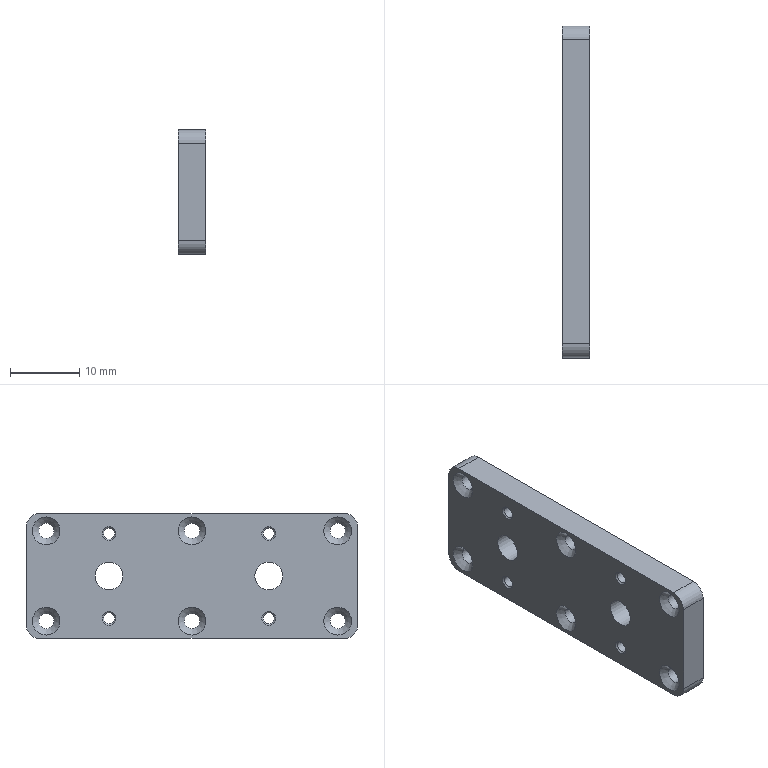Part | STEP file | Coupler cover | 1 solid | 36 faces | box 4 x 47.8 x 18 mm | volume 3182 mm3 | cylinder 16 | cone 14 | plane 6 | commonest cylinder face diameters 2.2 x6 4 x6 1.6 x4